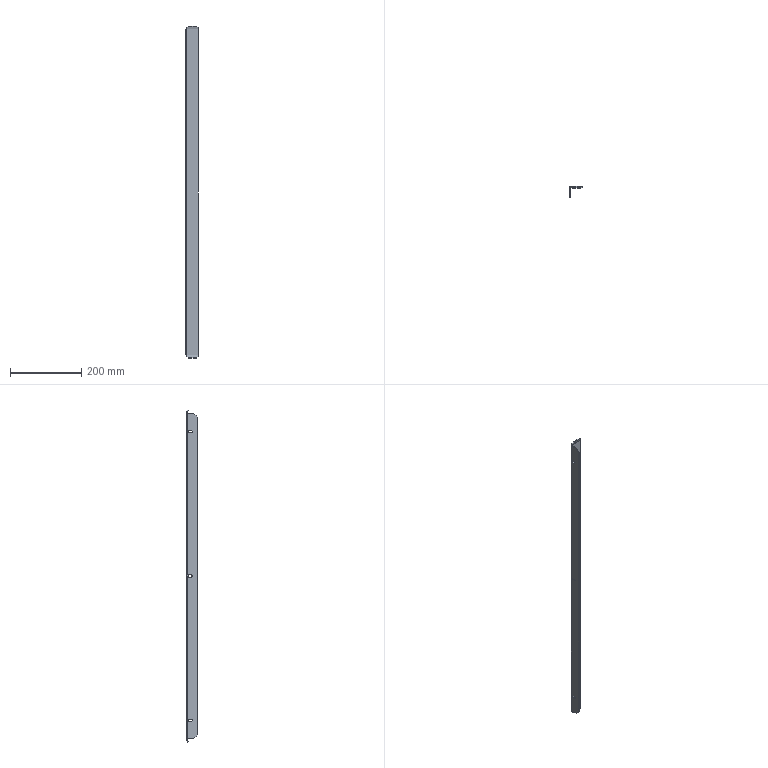Part | STEP file | BPSP-03-031Long Support Plate (Lower)_Default | 1 solid | 48 faces | box 35 x 30 x 929.978 mm | volume 113908 mm3 | plane 36 | cylinder 12 | commonest cylinder face diameters 6 x6 1.473 x3 5.473 x3